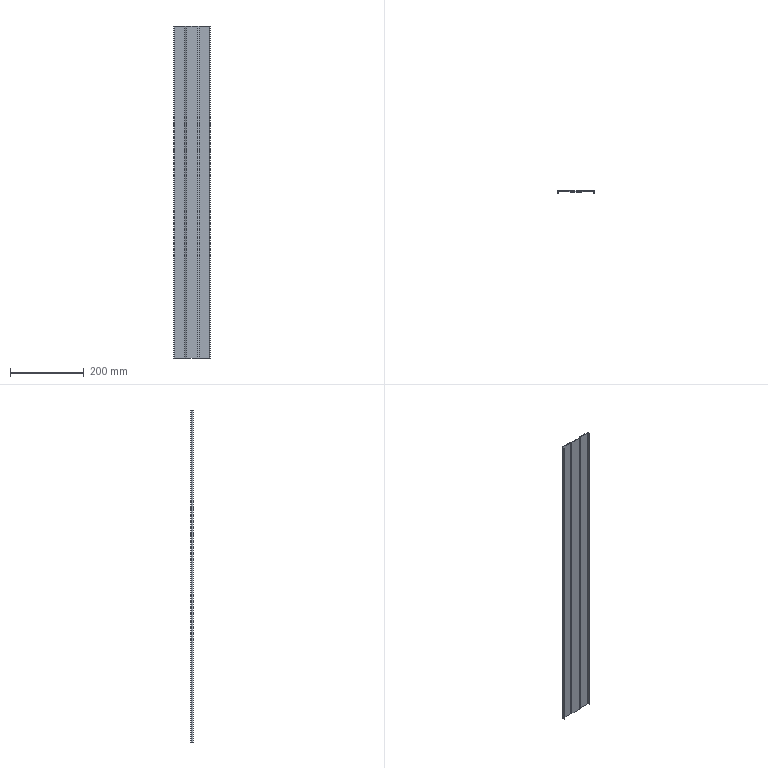Part | STEP file | Crossbeam front guard plate | 1 solid | 54 faces | box 98 x 8 x 898 mm | volume 149433 mm3 | plane 42 | cylinder 12 | commonest cylinder face diameters 1 x6 4 x6
STEP:
#1=CARTESIAN_POINT('',(98.,-2.,898.));
#2=VERTEX_POINT('',#1);
#3=CARTESIAN_POINT('',(96.5,-2.,898.));
#4=VERTEX_POINT('',#3);
#5=CARTESIAN_POINT('',(98.,-2.,898.));
#6=DIRECTION('',(-1.,0.,0.));
#7=VECTOR('',#6,1000.);
#8=LINE('',#5,#7);
#9=EDGE_CURVE('',#2,#4,#8,.T.);
#10=ORIENTED_EDGE('',*,*,#9,.F.);
#11=CARTESIAN_POINT('',(96.,0.,898.));
#12=VERTEX_POINT('',#11);
#13=CARTESIAN_POINT('',(96.,-2.,898.));
#14=DIRECTION('',(0.,0.,1.));
#15=DIRECTION('',(-1.,0.,0.));
#16=AXIS2_PLACEMENT_3D('',#13,#14,#15);
#17=CIRCLE('',#16,2.);
#18=EDGE_CURVE('',#2,#12,#17,.T.);
#19=ORIENTED_EDGE('',*,*,#18,.T.);
#20=CARTESIAN_POINT('',(96.,-1.5,898.));
#21=VERTEX_POINT('',#20);
#22=CARTESIAN_POINT('',(96.,-1.5,898.));
#23=DIRECTION('',(0.,1.,0.));
#24=VECTOR('',#23,1000.);
#25=LINE('',#22,#24);
#26=EDGE_CURVE('',#21,#12,#25,.T.);
#27=ORIENTED_EDGE('',*,*,#26,.F.);
#28=CARTESIAN_POINT('',(96.,-2.,898.));
#29=DIRECTION('',(0.,0.,1.));
#30=DIRECTION('',(1.,0.,0.));
#31=AXIS2_PLACEMENT_3D('',#28,#29,#30);
#32=CIRCLE('',#31,0.5);
#33=EDGE_CURVE('',#4,#21,#32,.T.);
#34=ORIENTED_EDGE('',*,*,#33,.F.);
#35=EDGE_LOOP('',(#10,#19,#27,#34));
#36=FACE_OUTER_BOUND('',#35,.T.);
#37=CARTESIAN_POINT('',(98.,-2.,898.));
#38=DIRECTION('',(0.,0.,1.));
#39=DIRECTION('',(1.,0.,0.));
#40=AXIS2_PLACEMENT_3D('',#37,#38,#39);
#41=PLANE('',#40);
#42=ADVANCED_FACE('',(#36),#41,.T.);
#43=CARTESIAN_POINT('',(98.,-8.,898.));
#44=VERTEX_POINT('',#43);
#45=CARTESIAN_POINT('',(98.,0.,898.));
#46=DIRECTION('',(0.,1.,0.));
#47=VECTOR('',#46,1000.);
#48=LINE('',#45,#47);
#49=EDGE_CURVE('',#44,#2,#48,.T.);
#50=ORIENTED_EDGE('',*,*,#49,.T.);
#51=ORIENTED_EDGE('',*,*,#9,.T.);
#52=CARTESIAN_POINT('',(96.5,-8.,898.));
#53=VERTEX_POINT('',#52);
#54=CARTESIAN_POINT('',(96.5,0.,898.));
#55=DIRECTION('',(0.,1.,0.));
#56=VECTOR('',#55,1000.);
#57=LINE('',#54,#56);
#58=EDGE_CURVE('',#53,#4,#57,.T.);
#59=ORIENTED_EDGE('',*,*,#58,.F.);
#60=CARTESIAN_POINT('',(98.,-8.,898.));
#61=DIRECTION('',(-1.,0.,0.));
#62=VECTOR('',#61,1000.);
#63=LINE('',#60,#62);
#64=EDGE_CURVE('',#44,#53,#63,.T.);
#65=ORIENTED_EDGE('',*,*,#64,.F.);
#66=EDGE_LOOP('',(#50,#51,#59,#65));
#67=FACE_OUTER_BOUND('',#66,.T.);
#68=CARTESIAN_POINT('',(96.,-1.5,898.));
#69=DIRECTION('',(0.,0.,1.));
#70=DIRECTION('',(1.,0.,0.));
#71=AXIS2_PLACEMENT_3D('',#68,#69,#70);
#72=PLANE('',#71);
#73=ADVANCED_FACE('',(#67),#72,.T.);
#74=CARTESIAN_POINT('',(96.,0.,0.));
#75=VERTEX_POINT('',#74);
#76=CARTESIAN_POINT('',(96.,-1.5,0.));
#77=VERTEX_POINT('',#76);
#78=CARTESIAN_POINT('',(96.,0.,0.));
#79=DIRECTION('',(0.,-1.,0.));
#80=VECTOR('',#79,1000.);
#81=LINE('',#78,#80);
#82=EDGE_CURVE('',#75,#77,#81,.T.);
#83=ORIENTED_EDGE('',*,*,#82,.F.);
#84=CARTESIAN_POINT('',(98.,-2.,0.));
#85=VERTEX_POINT('',#84);
#86=CARTESIAN_POINT('',(96.,-2.,0.));
#87=DIRECTION('',(0.,0.,1.));
#88=DIRECTION('',(-1.,0.,0.));
#89=AXIS2_PLACEMENT_3D('',#86,#87,#88);
#90=CIRCLE('',#89,2.);
#91=EDGE_CURVE('',#85,#75,#90,.T.);
#92=ORIENTED_EDGE('',*,*,#91,.F.);
#93=CARTESIAN_POINT('',(96.5,-2.,0.));
#94=VERTEX_POINT('',#93);
#95=CARTESIAN_POINT('',(96.5,-2.,0.));
#96=DIRECTION('',(1.,0.,0.));
#97=VECTOR('',#96,1000.);
#98=LINE('',#95,#97);
#99=EDGE_CURVE('',#94,#85,#98,.T.);
#100=ORIENTED_EDGE('',*,*,#99,.F.);
#101=CARTESIAN_POINT('',(96.,-2.,0.));
#102=DIRECTION('',(0.,0.,1.));
#103=DIRECTION('',(1.,0.,0.));
#104=AXIS2_PLACEMENT_3D('',#101,#102,#103);
#105=CIRCLE('',#104,0.5);
#106=EDGE_CURVE('',#94,#77,#105,.T.);
#107=ORIENTED_EDGE('',*,*,#106,.T.);
#108=EDGE_LOOP('',(#83,#92,#100,#107));
#109=FACE_OUTER_BOUND('',#108,.T.);
#110=CARTESIAN_POINT('',(96.,0.,0.));
#111=DIRECTION('',(0.,0.,-1.));
#112=DIRECTION('',(-1.,0.,0.));
#113=AXIS2_PLACEMENT_3D('',#110,#111,#112);
#114=PLANE('',#113);
#115=ADVANCED_FACE('',(#109),#114,.T.);
#116=CARTESIAN_POINT('',(68.,0.,0.));
#117=VERTEX_POINT('',#116);
#118=CARTESIAN_POINT('',(67.464,0.,0.));
#119=DIRECTION('',(-1.,0.,0.));
#120=VECTOR('',#119,1000.);
#121=LINE('',#118,#120);
#122=EDGE_CURVE('',#75,#117,#121,.T.);
#123=ORIENTED_EDGE('',*,*,#122,.F.);
#124=ORIENTED_EDGE('',*,*,#82,.T.);
#125=CARTESIAN_POINT('',(68.,-1.5,0.));
#126=VERTEX_POINT('',#125);
#127=CARTESIAN_POINT('',(67.464,-1.5,0.));
#128=DIRECTION('',(-1.,0.,0.));
#129=VECTOR('',#128,1000.);
#130=LINE('',#127,#129);
#131=EDGE_CURVE('',#77,#126,#130,.T.);
#132=ORIENTED_EDGE('',*,*,#131,.T.);
#133=CARTESIAN_POINT('',(68.,-1.5,0.));
#134=DIRECTION('',(0.,1.,0.));
#135=VECTOR('',#134,1000.);
#136=LINE('',#133,#135);
#137=EDGE_CURVE('',#126,#117,#136,.T.);
#138=ORIENTED_EDGE('',*,*,#137,.T.);
#139=EDGE_LOOP('',(#123,#124,#132,#138));
#140=FACE_OUTER_BOUND('',#139,.T.);
#141=CARTESIAN_POINT('',(96.5,-2.,0.));
#142=DIRECTION('',(0.,0.,-1.));
#143=DIRECTION('',(-1.,0.,0.));
#144=AXIS2_PLACEMENT_3D('',#141,#142,#143);
#145=PLANE('',#144);
#146=ADVANCED_FACE('',(#140),#145,.T.);
#147=CARTESIAN_POINT('',(68.,0.,898.));
#148=VERTEX_POINT('',#147);
#149=CARTESIAN_POINT('',(68.,-1.5,898.));
#150=VERTEX_POINT('',#149);
#151=CARTESIAN_POINT('',(68.,0.,898.));
#152=DIRECTION('',(0.,-1.,0.));
#153=VECTOR('',#152,1000.);
#154=LINE('',#151,#153);
#155=EDGE_CURVE('',#148,#150,#154,.T.);
#156=ORIENTED_EDGE('',*,*,#155,.F.);
#157=CARTESIAN_POINT('',(67.,-0.2679,898.));
#158=VERTEX_POINT('',#157);
#159=CARTESIAN_POINT('',(68.,-2.,898.));
#160=DIRECTION('',(0.,0.,1.));
#161=DIRECTION('',(-1.,0.,0.));
#162=AXIS2_PLACEMENT_3D('',#159,#160,#161);
#163=CIRCLE('',#162,2.);
#164=EDGE_CURVE('',#148,#158,#163,.T.);
#165=ORIENTED_EDGE('',*,*,#164,.T.);
#166=CARTESIAN_POINT('',(67.75,-1.567,898.));
#167=VERTEX_POINT('',#166);
#168=CARTESIAN_POINT('',(67.75,-1.567,898.));
#169=DIRECTION('',(-0.5,0.866,0.));
#170=VECTOR('',#169,1000.);
#171=LINE('',#168,#170);
#172=EDGE_CURVE('',#167,#158,#171,.T.);
#173=ORIENTED_EDGE('',*,*,#172,.F.);
#174=CARTESIAN_POINT('',(68.,-2.,898.));
#175=DIRECTION('',(0.,0.,1.));
#176=DIRECTION('',(1.,0.,0.));
#177=AXIS2_PLACEMENT_3D('',#174,#175,#176);
#178=CIRCLE('',#177,0.5);
#179=EDGE_CURVE('',#150,#167,#178,.T.);
#180=ORIENTED_EDGE('',*,*,#179,.F.);
#181=EDGE_LOOP('',(#156,#165,#173,#180));
#182=FACE_OUTER_BOUND('',#181,.T.);
#183=CARTESIAN_POINT('',(68.,0.,898.));
#184=DIRECTION('',(0.,0.,1.));
#185=DIRECTION('',(1.,0.,0.));
#186=AXIS2_PLACEMENT_3D('',#183,#184,#185);
#187=PLANE('',#186);
#188=ADVANCED_FACE('',(#182),#187,.T.);
#189=CARTESIAN_POINT('',(67.464,0.,898.));
#190=DIRECTION('',(-1.,0.,0.));
#191=VECTOR('',#190,1000.);
#192=LINE('',#189,#191);
#193=EDGE_CURVE('',#12,#148,#192,.T.);
#194=ORIENTED_EDGE('',*,*,#193,.T.);
#195=ORIENTED_EDGE('',*,*,#155,.T.);
#196=CARTESIAN_POINT('',(67.464,-1.5,898.));
#197=DIRECTION('',(-1.,0.,0.));
#198=VECTOR('',#197,1000.);
#199=LINE('',#196,#198);
#200=EDGE_CURVE('',#21,#150,#199,.T.);
#201=ORIENTED_EDGE('',*,*,#200,.F.);
#202=ORIENTED_EDGE('',*,*,#26,.T.);
#203=EDGE_LOOP('',(#194,#195,#201,#202));
#204=FACE_OUTER_BOUND('',#203,.T.);
#205=CARTESIAN_POINT('',(67.75,-1.567,898.));
#206=DIRECTION('',(0.,0.,1.));
#207=DIRECTION('',(1.,0.,0.));
#208=AXIS2_PLACEMENT_3D('',#205,#206,#207);
#209=PLANE('',#208);
#210=ADVANCED_FACE('',(#204),#209,.T.);
#211=CARTESIAN_POINT('',(67.,-0.2679,0.));
#212=VERTEX_POINT('',#211);
#213=CARTESIAN_POINT('',(67.75,-1.567,0.));
#214=VERTEX_POINT('',#213);
#215=CARTESIAN_POINT('',(67.,-0.2679,0.));
#216=DIRECTION('',(0.5,-0.866,0.));
#217=VECTOR('',#216,1000.);
#218=LINE('',#215,#217);
#219=EDGE_CURVE('',#212,#214,#218,.T.);
#220=ORIENTED_EDGE('',*,*,#219,.F.);
#221=CARTESIAN_POINT('',(68.,-2.,0.));
#222=DIRECTION('',(0.,0.,1.));
#223=DIRECTION('',(-1.,0.,0.));
#224=AXIS2_PLACEMENT_3D('',#221,#222,#223);
#225=CIRCLE('',#224,2.);
#226=EDGE_CURVE('',#117,#212,#225,.T.);
#227=ORIENTED_EDGE('',*,*,#226,.F.);
#228=ORIENTED_EDGE('',*,*,#137,.F.);
#229=CARTESIAN_POINT('',(68.,-2.,0.));
#230=DIRECTION('',(0.,0.,1.));
#231=DIRECTION('',(1.,0.,0.));
#232=AXIS2_PLACEMENT_3D('',#229,#230,#231);
#233=CIRCLE('',#232,0.5);
#234=EDGE_CURVE('',#126,#214,#233,.T.);
#235=ORIENTED_EDGE('',*,*,#234,.T.);
#236=EDGE_LOOP('',(#220,#227,#228,#235));
#237=FACE_OUTER_BOUND('',#236,.T.);
#238=CARTESIAN_POINT('',(67.,-0.2679,0.));
#239=DIRECTION('',(0.,0.,-1.));
#240=DIRECTION('',(-1.,0.,0.));
#241=AXIS2_PLACEMENT_3D('',#238,#239,#240);
#242=PLANE('',#241);
#243=ADVANCED_FACE('',(#237),#242,.T.);
#244=CARTESIAN_POINT('',(64.116,-1.933,0.));
#245=VERTEX_POINT('',#244);
#246=CARTESIAN_POINT('',(64.,-2.,0.));
#247=DIRECTION('',(-0.866,-0.5,0.));
#248=VECTOR('',#247,1000.);
#249=LINE('',#246,#248);
#250=EDGE_CURVE('',#212,#245,#249,.T.);
#251=ORIENTED_EDGE('',*,*,#250,.F.);
#252=ORIENTED_EDGE('',*,*,#219,.T.);
#253=CARTESIAN_POINT('',(64.866,-3.232,0.));
#254=VERTEX_POINT('',#253);
#255=CARTESIAN_POINT('',(64.75,-3.299,0.));
#256=DIRECTION('',(-0.866,-0.5,0.));
#257=VECTOR('',#256,1000.);
#258=LINE('',#255,#257);
#259=EDGE_CURVE('',#214,#254,#258,.T.);
#260=ORIENTED_EDGE('',*,*,#259,.T.);
#261=CARTESIAN_POINT('',(64.866,-3.232,0.));
#262=DIRECTION('',(-0.5,0.866,0.));
#263=VECTOR('',#262,1000.);
#264=LINE('',#261,#263);
#265=EDGE_CURVE('',#254,#245,#264,.T.);
#266=ORIENTED_EDGE('',*,*,#265,.T.);
#267=EDGE_LOOP('',(#251,#252,#260,#266));
#268=FACE_OUTER_BOUND('',#267,.T.);
#269=CARTESIAN_POINT('',(68.,-1.5,0.));
#270=DIRECTION('',(0.,0.,-1.));
#271=DIRECTION('',(-1.,0.,0.));
#272=AXIS2_PLACEMENT_3D('',#269,#270,#271);
#273=PLANE('',#272);
#274=ADVANCED_FACE('',(#268),#273,.T.);
#275=CARTESIAN_POINT('',(64.116,-1.933,898.));
#276=VERTEX_POINT('',#275);
#277=CARTESIAN_POINT('',(64.866,-3.232,898.));
#278=VERTEX_POINT('',#277);
#279=CARTESIAN_POINT('',(64.116,-1.933,898.));
#280=DIRECTION('',(0.5,-0.866,0.));
#281=VECTOR('',#280,1000.);
#282=LINE('',#279,#281);
#283=EDGE_CURVE('',#276,#278,#282,.T.);
#284=ORIENTED_EDGE('',*,*,#283,.F.);
#285=CARTESIAN_POINT('',(63.866,-2.,898.));
#286=VERTEX_POINT('',#285);
#287=CARTESIAN_POINT('',(63.866,-1.5,898.));
#288=DIRECTION('',(0.,0.,-1.));
#289=DIRECTION('',(1.,0.,0.));
#290=AXIS2_PLACEMENT_3D('',#287,#288,#289);
#291=CIRCLE('',#290,0.5);
#292=EDGE_CURVE('',#276,#286,#291,.T.);
#293=ORIENTED_EDGE('',*,*,#292,.T.);
#294=CARTESIAN_POINT('',(63.866,-3.5,898.));
#295=VERTEX_POINT('',#294);
#296=CARTESIAN_POINT('',(63.866,-3.5,898.));
#297=DIRECTION('',(0.,1.,0.));
#298=VECTOR('',#297,1000.);
#299=LINE('',#296,#298);
#300=EDGE_CURVE('',#295,#286,#299,.T.);
#301=ORIENTED_EDGE('',*,*,#300,.F.);
#302=CARTESIAN_POINT('',(63.866,-1.5,898.));
#303=DIRECTION('',(0.,0.,-1.));
#304=DIRECTION('',(1.,0.,0.));
#305=AXIS2_PLACEMENT_3D('',#302,#303,#304);
#306=CIRCLE('',#305,2.);
#307=EDGE_CURVE('',#278,#295,#306,.T.);
#308=ORIENTED_EDGE('',*,*,#307,.F.);
#309=EDGE_LOOP('',(#284,#293,#301,#308));
#310=FACE_OUTER_BOUND('',#309,.T.);
#311=CARTESIAN_POINT('',(64.116,-1.933,898.));
#312=DIRECTION('',(0.,0.,1.));
#313=DIRECTION('',(1.,0.,0.));
#314=AXIS2_PLACEMENT_3D('',#311,#312,#313);
#315=PLANE('',#314);
#316=ADVANCED_FACE('',(#310),#315,.T.);
#317=CARTESIAN_POINT('',(64.,-2.,898.));
#318=DIRECTION('',(-0.866,-0.5,0.));
#319=VECTOR('',#318,1000.);
#320=LINE('',#317,#319);
#321=EDGE_CURVE('',#158,#276,#320,.T.);
#322=ORIENTED_EDGE('',*,*,#321,.T.);
#323=ORIENTED_EDGE('',*,*,#283,.T.);
#324=CARTESIAN_POINT('',(64.75,-3.299,898.));
#325=DIRECTION('',(-0.866,-0.5,0.));
#326=VECTOR('',#325,1000.);
#327=LINE('',#324,#326);
#328=EDGE_CURVE('',#167,#278,#327,.T.);
#329=ORIENTED_EDGE('',*,*,#328,.F.);
#330=ORIENTED_EDGE('',*,*,#172,.T.);
#331=EDGE_LOOP('',(#322,#323,#329,#330));
#332=FACE_OUTER_BOUND('',#331,.T.);
#333=CARTESIAN_POINT('',(63.866,-3.5,898.));
#334=DIRECTION('',(0.,0.,1.));
#335=DIRECTION('',(1.,0.,0.));
#336=AXIS2_PLACEMENT_3D('',#333,#334,#335);
#337=PLANE('',#336);
#338=ADVANCED_FACE('',(#332),#337,.T.);
#339=CARTESIAN_POINT('',(63.866,-2.,0.));
#340=VERTEX_POINT('',#339);
#341=CARTESIAN_POINT('',(63.866,-3.5,0.));
#342=VERTEX_POINT('',#341);
#343=CARTESIAN_POINT('',(63.866,-2.,0.));
#344=DIRECTION('',(0.,-1.,0.));
#345=VECTOR('',#344,1000.);
#346=LINE('',#343,#345);
#347=EDGE_CURVE('',#340,#342,#346,.T.);
#348=ORIENTED_EDGE('',*,*,#347,.F.);
#349=CARTESIAN_POINT('',(63.866,-1.5,0.));
#350=DIRECTION('',(0.,0.,-1.));
#351=DIRECTION('',(1.,0.,0.));
#352=AXIS2_PLACEMENT_3D('',#349,#350,#351);
#353=CIRCLE('',#352,0.5);
#354=EDGE_CURVE('',#245,#340,#353,.T.);
#355=ORIENTED_EDGE('',*,*,#354,.F.);
#356=ORIENTED_EDGE('',*,*,#265,.F.);
#357=CARTESIAN_POINT('',(63.866,-1.5,0.));
#358=DIRECTION('',(0.,0.,-1.));
#359=DIRECTION('',(1.,0.,0.));
#360=AXIS2_PLACEMENT_3D('',#357,#358,#359);
#361=CIRCLE('',#360,2.);
#362=EDGE_CURVE('',#254,#342,#361,.T.);
#363=ORIENTED_EDGE('',*,*,#362,.T.);
#364=EDGE_LOOP('',(#348,#355,#356,#363));
#365=FACE_OUTER_BOUND('',#364,.T.);
#366=CARTESIAN_POINT('',(63.866,-2.,0.));
#367=DIRECTION('',(0.,0.,-1.));
#368=DIRECTION('',(-1.,0.,0.));
#369=AXIS2_PLACEMENT_3D('',#366,#367,#368);
#370=PLANE('',#369);
#371=ADVANCED_FACE('',(#365),#370,.T.);
#372=CARTESIAN_POINT('',(34.134,-2.,0.));
#373=VERTEX_POINT('',#372);
#374=CARTESIAN_POINT('',(34.,-2.,0.));
#375=DIRECTION('',(-1.,0.,0.));
#376=VECTOR('',#375,1000.);
#377=LINE('',#374,#376);
#378=EDGE_CURVE('',#340,#373,#377,.T.);
#379=ORIENTED_EDGE('',*,*,#378,.F.);
#380=ORIENTED_EDGE('',*,*,#347,.T.);
#381=CARTESIAN_POINT('',(34.134,-3.5,0.));
#382=VERTEX_POINT('',#381);
#383=CARTESIAN_POINT('',(34.,-3.5,0.));
#384=DIRECTION('',(-1.,0.,0.));
#385=VECTOR('',#384,1000.);
#386=LINE('',#383,#385);
#387=EDGE_CURVE('',#342,#382,#386,.T.);
#388=ORIENTED_EDGE('',*,*,#387,.T.);
#389=CARTESIAN_POINT('',(34.134,-3.5,0.));
#390=DIRECTION('',(0.,1.,0.));
#391=VECTOR('',#390,1000.);
#392=LINE('',#389,#391);
#393=EDGE_CURVE('',#382,#373,#392,.T.);
#394=ORIENTED_EDGE('',*,*,#393,.T.);
#395=EDGE_LOOP('',(#379,#380,#388,#394));
#396=FACE_OUTER_BOUND('',#395,.T.);
#397=CARTESIAN_POINT('',(64.866,-3.232,0.));
#398=DIRECTION('',(0.,0.,-1.));
#399=DIRECTION('',(-1.,0.,0.));
#400=AXIS2_PLACEMENT_3D('',#397,#398,#399);
#401=PLANE('',#400);
#402=ADVANCED_FACE('',(#396),#401,.T.);
#403=CARTESIAN_POINT('',(34.134,-2.,898.));
#404=VERTEX_POINT('',#403);
#405=CARTESIAN_POINT('',(34.134,-3.5,898.));
#406=VERTEX_POINT('',#405);
#407=CARTESIAN_POINT('',(34.134,-2.,898.));
#408=DIRECTION('',(0.,-1.,0.));
#409=VECTOR('',#408,1000.);
#410=LINE('',#407,#409);
#411=EDGE_CURVE('',#404,#406,#410,.T.);
#412=ORIENTED_EDGE('',*,*,#411,.F.);
#413=CARTESIAN_POINT('',(33.884,-1.933,898.));
#414=VERTEX_POINT('',#413);
#415=CARTESIAN_POINT('',(34.134,-1.5,898.));
#416=DIRECTION('',(0.,0.,-1.));
#417=DIRECTION('',(1.,0.,0.));
#418=AXIS2_PLACEMENT_3D('',#415,#416,#417);
#419=CIRCLE('',#418,0.5);
#420=EDGE_CURVE('',#404,#414,#419,.T.);
#421=ORIENTED_EDGE('',*,*,#420,.T.);
#422=CARTESIAN_POINT('',(33.134,-3.232,898.));
#423=VERTEX_POINT('',#422);
#424=CARTESIAN_POINT('',(33.134,-3.232,898.));
#425=DIRECTION('',(0.5,0.866,0.));
#426=VECTOR('',#425,1000.);
#427=LINE('',#424,#426);
#428=EDGE_CURVE('',#423,#414,#427,.T.);
#429=ORIENTED_EDGE('',*,*,#428,.F.);
#430=CARTESIAN_POINT('',(34.134,-1.5,898.));
#431=DIRECTION('',(0.,0.,-1.));
#432=DIRECTION('',(1.,0.,0.));
#433=AXIS2_PLACEMENT_3D('',#430,#431,#432);
#434=CIRCLE('',#433,2.);
#435=EDGE_CURVE('',#406,#423,#434,.T.);
#436=ORIENTED_EDGE('',*,*,#435,.F.);
#437=EDGE_LOOP('',(#412,#421,#429,#436));
#438=FACE_OUTER_BOUND('',#437,.T.);
#439=CARTESIAN_POINT('',(34.134,-2.,898.));
#440=DIRECTION('',(0.,0.,1.));
#441=DIRECTION('',(1.,0.,0.));
#442=AXIS2_PLACEMENT_3D('',#439,#440,#441);
#443=PLANE('',#442);
#444=ADVANCED_FACE('',(#438),#443,.T.);
#445=CARTESIAN_POINT('',(34.,-2.,898.));
#446=DIRECTION('',(-1.,0.,0.));
#447=VECTOR('',#446,1000.);
#448=LINE('',#445,#447);
#449=EDGE_CURVE('',#286,#404,#448,.T.);
#450=ORIENTED_EDGE('',*,*,#449,.T.);
#451=ORIENTED_EDGE('',*,*,#411,.T.);
#452=CARTESIAN_POINT('',(34.,-3.5,898.));
#453=DIRECTION('',(-1.,0.,0.));
#454=VECTOR('',#453,1000.);
#455=LINE('',#452,#454);
#456=EDGE_CURVE('',#295,#406,#455,.T.);
#457=ORIENTED_EDGE('',*,*,#456,.F.);
#458=ORIENTED_EDGE('',*,*,#300,.T.);
#459=EDGE_LOOP('',(#450,#451,#457,#458));
#460=FACE_OUTER_BOUND('',#459,.T.);
#461=CARTESIAN_POINT('',(33.134,-3.232,898.));
#462=DIRECTION('',(0.,0.,1.));
#463=DIRECTION('',(1.,0.,0.));
#464=AXIS2_PLACEMENT_3D('',#461,#462,#463);
#465=PLANE('',#464);
#466=ADVANCED_FACE('',(#460),#465,.T.);
#467=CARTESIAN_POINT('',(33.884,-1.933,0.));
#468=VERTEX_POINT('',#467);
#469=CARTESIAN_POINT('',(33.134,-3.232,0.));
#470=VERTEX_POINT('',#469);
#471=CARTESIAN_POINT('',(33.884,-1.933,0.));
#472=DIRECTION('',(-0.5,-0.866,0.));
#473=VECTOR('',#472,1000.);
#474=LINE('',#471,#473);
#475=EDGE_CURVE('',#468,#470,#474,.T.);
#476=ORIENTED_EDGE('',*,*,#475,.F.);
#477=CARTESIAN_POINT('',(34.134,-1.5,0.));
#478=DIRECTION('',(0.,0.,-1.));
#479=DIRECTION('',(1.,0.,0.));
#480=AXIS2_PLACEMENT_3D('',#477,#478,#479);
#481=CIRCLE('',#480,0.5);
#482=EDGE_CURVE('',#373,#468,#481,.T.);
#483=ORIENTED_EDGE('',*,*,#482,.F.);
#484=ORIENTED_EDGE('',*,*,#393,.F.);
#485=CARTESIAN_POINT('',(34.134,-1.5,0.));
#486=DIRECTION('',(0.,0.,-1.));
#487=DIRECTION('',(1.,0.,0.));
#488=AXIS2_PLACEMENT_3D('',#485,#486,#487);
#489=CIRCLE('',#488,2.);
#490=EDGE_CURVE('',#382,#470,#489,.T.);
#491=ORIENTED_EDGE('',*,*,#490,.T.);
#492=EDGE_LOOP('',(#476,#483,#484,#491));
#493=FACE_OUTER_BOUND('',#492,.T.);
#494=CARTESIAN_POINT('',(33.884,-1.933,0.));
#495=DIRECTION('',(0.,0.,-1.));
#496=DIRECTION('',(-1.,0.,0.));
#497=AXIS2_PLACEMENT_3D('',#494,#495,#496);
#498=PLANE('',#497);
#499=ADVANCED_FACE('',(#493),#498,.T.);
#500=CARTESIAN_POINT('',(31.,-0.2679,0.));
#501=VERTEX_POINT('',#500);
#502=CARTESIAN_POINT('',(30.536,0.,0.));
#503=DIRECTION('',(-0.866,0.5,0.));
#504=VECTOR('',#503,1000.);
#505=LINE('',#502,#504);
#506=EDGE_CURVE('',#468,#501,#505,.T.);
#507=ORIENTED_EDGE('',*,*,#506,.F.);
#508=ORIENTED_EDGE('',*,*,#475,.T.);
#509=CARTESIAN_POINT('',(30.25,-1.567,0.));
#510=VERTEX_POINT('',#509);
#511=CARTESIAN_POINT('',(29.786,-1.299,0.));
#512=DIRECTION('',(-0.866,0.5,0.));
#513=VECTOR('',#512,1000.);
#514=LINE('',#511,#513);
#515=EDGE_CURVE('',#470,#510,#514,.T.);
#516=ORIENTED_EDGE('',*,*,#515,.T.);
#517=CARTESIAN_POINT('',(30.25,-1.567,0.));
#518=DIRECTION('',(0.5,0.866,0.));
#519=VECTOR('',#518,1000.);
#520=LINE('',#517,#519);
#521=EDGE_CURVE('',#510,#501,#520,.T.);
#522=ORIENTED_EDGE('',*,*,#521,.T.);
#523=EDGE_LOOP('',(#507,#508,#516,#522));
#524=FACE_OUTER_BOUND('',#523,.T.);
#525=CARTESIAN_POINT('',(34.134,-3.5,0.));
#526=DIRECTION('',(0.,0.,-1.));
#527=DIRECTION('',(-1.,0.,0.));
#528=AXIS2_PLACEMENT_3D('',#525,#526,#527);
#529=PLANE('',#528);
#530=ADVANCED_FACE('',(#524),#529,.T.);
#531=CARTESIAN_POINT('',(31.,-0.2679,898.));
#532=VERTEX_POINT('',#531);
#533=CARTESIAN_POINT('',(30.25,-1.567,898.));
#534=VERTEX_POINT('',#533);
#535=CARTESIAN_POINT('',(31.,-0.2679,898.));
#536=DIRECTION('',(-0.5,-0.866,0.));
#537=VECTOR('',#536,1000.);
#538=LINE('',#535,#537);
#539=EDGE_CURVE('',#532,#534,#538,.T.);
#540=ORIENTED_EDGE('',*,*,#539,.F.);
#541=CARTESIAN_POINT('',(30.,0.,898.));
#542=VERTEX_POINT('',#541);
#543=CARTESIAN_POINT('',(30.,-2.,898.));
#544=DIRECTION('',(0.,0.,1.));
#545=DIRECTION('',(-1.,0.,0.));
#546=AXIS2_PLACEMENT_3D('',#543,#544,#545);
#547=CIRCLE('',#546,2.);
#548=EDGE_CURVE('',#532,#542,#547,.T.);
#549=ORIENTED_EDGE('',*,*,#548,.T.);
#550=CARTESIAN_POINT('',(30.,-1.5,898.));
#551=VERTEX_POINT('',#550);
#552=CARTESIAN_POINT('',(30.,-1.5,898.));
#553=DIRECTION('',(0.,1.,0.));
#554=VECTOR('',#553,1000.);
#555=LINE('',#552,#554);
#556=EDGE_CURVE('',#551,#542,#555,.T.);
#557=ORIENTED_EDGE('',*,*,#556,.F.);
#558=CARTESIAN_POINT('',(30.,-2.,898.));
#559=DIRECTION('',(0.,0.,1.));
#560=DIRECTION('',(1.,0.,0.));
#561=AXIS2_PLACEMENT_3D('',#558,#559,#560);
#562=CIRCLE('',#561,0.5);
#563=EDGE_CURVE('',#534,#551,#562,.T.);
#564=ORIENTED_EDGE('',*,*,#563,.F.);
#565=EDGE_LOOP('',(#540,#549,#557,#564));
#566=FACE_OUTER_BOUND('',#565,.T.);
#567=CARTESIAN_POINT('',(31.,-0.2679,898.));
#568=DIRECTION('',(0.,0.,1.));
#569=DIRECTION('',(1.,0.,0.));
#570=AXIS2_PLACEMENT_3D('',#567,#568,#569);
#571=PLANE('',#570);
#572=ADVANCED_FACE('',(#566),#571,.T.);
#573=CARTESIAN_POINT('',(30.536,0.,898.));
#574=DIRECTION('',(-0.866,0.5,0.));
#575=VECTOR('',#574,1000.);
#576=LINE('',#573,#575);
#577=EDGE_CURVE('',#414,#532,#576,.T.);
#578=ORIENTED_EDGE('',*,*,#577,.T.);
#579=ORIENTED_EDGE('',*,*,#539,.T.);
#580=CARTESIAN_POINT('',(29.786,-1.299,898.));
#581=DIRECTION('',(-0.866,0.5,0.));
#582=VECTOR('',#581,1000.);
#583=LINE('',#580,#582);
#584=EDGE_CURVE('',#423,#534,#583,.T.);
#585=ORIENTED_EDGE('',*,*,#584,.F.);
#586=ORIENTED_EDGE('',*,*,#428,.T.);
#587=EDGE_LOOP('',(#578,#579,#585,#586));
#588=FACE_OUTER_BOUND('',#587,.T.);
#589=CARTESIAN_POINT('',(30.,-1.5,898.));
#590=DIRECTION('',(0.,0.,1.));
#591=DIRECTION('',(1.,0.,0.));
#592=AXIS2_PLACEMENT_3D('',#589,#590,#591);
#593=PLANE('',#592);
#594=ADVANCED_FACE('',(#588),#593,.T.);
#595=CARTESIAN_POINT('',(30.,0.,0.));
#596=VERTEX_POINT('',#595);
#597=CARTESIAN_POINT('',(30.,-1.5,0.));
#598=VERTEX_POINT('',#597);
#599=CARTESIAN_POINT('',(30.,0.,0.));
#600=DIRECTION('',(0.,-1.,0.));
#601=VECTOR('',#600,1000.);
#602=LINE('',#599,#601);
#603=EDGE_CURVE('',#596,#598,#602,.T.);
#604=ORIENTED_EDGE('',*,*,#603,.F.);
#605=CARTESIAN_POINT('',(30.,-2.,0.));
#606=DIRECTION('',(0.,0.,1.));
#607=DIRECTION('',(-1.,0.,0.));
#608=AXIS2_PLACEMENT_3D('',#605,#606,#607);
#609=CIRCLE('',#608,2.);
#610=EDGE_CURVE('',#501,#596,#609,.T.);
#611=ORIENTED_EDGE('',*,*,#610,.F.);
#612=ORIENTED_EDGE('',*,*,#521,.F.);
#613=CARTESIAN_POINT('',(30.,-2.,0.));
#614=DIRECTION('',(0.,0.,1.));
#615=DIRECTION('',(1.,0.,0.));
#616=AXIS2_PLACEMENT_3D('',#613,#614,#615);
#617=CIRCLE('',#616,0.5);
#618=EDGE_CURVE('',#510,#598,#617,.T.);
#619=ORIENTED_EDGE('',*,*,#618,.T.);
#620=EDGE_LOOP('',(#604,#611,#612,#619));
#621=FACE_OUTER_BOUND('',#620,.T.);
#622=CARTESIAN_POINT('',(30.,0.,0.));
#623=DIRECTION('',(0.,0.,-1.));
#624=DIRECTION('',(-1.,0.,0.));
#625=AXIS2_PLACEMENT_3D('',#622,#623,#624);
#626=PLANE('',#625);
#627=ADVANCED_FACE('',(#621),#626,.T.);
#628=CARTESIAN_POINT('',(2.,0.,0.));
#629=VERTEX_POINT('',#628);
#630=CARTESIAN_POINT('',(0.,0.,0.));
#631=DIRECTION('',(-1.,0.,0.));
#632=VECTOR('',#631,1000.);
#633=LINE('',#630,#632);
#634=EDGE_CURVE('',#596,#629,#633,.T.);
#635=ORIENTED_EDGE('',*,*,#634,.F.);
#636=ORIENTED_EDGE('',*,*,#603,.T.);
#637=CARTESIAN_POINT('',(2.,-1.5,0.));
#638=VERTEX_POINT('',#637);
#639=CARTESIAN_POINT('',(0.,-1.5,0.));
#640=DIRECTION('',(-1.,0.,0.));
#641=VECTOR('',#640,1000.);
#642=LINE('',#639,#641);
#643=EDGE_CURVE('',#598,#638,#642,.T.);
#644=ORIENTED_EDGE('',*,*,#643,.T.);
#645=CARTESIAN_POINT('',(2.,-1.5,0.));
#646=DIRECTION('',(0.,1.,0.));
#647=VECTOR('',#646,1000.);
#648=LINE('',#645,#647);
#649=EDGE_CURVE('',#638,#629,#648,.T.);
#650=ORIENTED_EDGE('',*,*,#649,.T.);
#651=EDGE_LOOP('',(#635,#636,#644,#650));
#652=FACE_OUTER_BOUND('',#651,.T.);
#653=CARTESIAN_POINT('',(30.25,-1.567,0.));
#654=DIRECTION('',(0.,0.,-1.));
#655=DIRECTION('',(-1.,0.,0.));
#656=AXIS2_PLACEMENT_3D('',#653,#654,#655);
#657=PLANE('',#656);
#658=ADVANCED_FACE('',(#652),#657,.T.);
#659=CARTESIAN_POINT('',(2.,0.,898.));
#660=VERTEX_POINT('',#659);
#661=CARTESIAN_POINT('',(2.,-1.5,898.));
#662=VERTEX_POINT('',#661);
#663=CARTESIAN_POINT('',(2.,0.,898.));
#664=DIRECTION('',(0.,-1.,0.));
#665=VECTOR('',#664,1000.);
#666=LINE('',#663,#665);
#667=EDGE_CURVE('',#660,#662,#666,.T.);
#668=ORIENTED_EDGE('',*,*,#667,.F.);
#669=CARTESIAN_POINT('',(0.,-2.,898.));
#670=VERTEX_POINT('',#669);
#671=CARTESIAN_POINT('',(2.,-2.,898.));
#672=DIRECTION('',(0.,0.,1.));
#673=DIRECTION('',(-1.,0.,0.));
#674=AXIS2_PLACEMENT_3D('',#671,#672,#673);
#675=CIRCLE('',#674,2.);
#676=EDGE_CURVE('',#660,#670,#675,.T.);
#677=ORIENTED_EDGE('',*,*,#676,.T.);
#678=CARTESIAN_POINT('',(1.5,-2.,898.));
#679=VERTEX_POINT('',#678);
#680=CARTESIAN_POINT('',(1.5,-2.,898.));
#681=DIRECTION('',(-1.,0.,0.));
#682=VECTOR('',#681,1000.);
#683=LINE('',#680,#682);
#684=EDGE_CURVE('',#679,#670,#683,.T.);
#685=ORIENTED_EDGE('',*,*,#684,.F.);
#686=CARTESIAN_POINT('',(2.,-2.,898.));
#687=DIRECTION('',(0.,0.,1.));
#688=DIRECTION('',(1.,0.,0.));
#689=AXIS2_PLACEMENT_3D('',#686,#687,#688);
#690=CIRCLE('',#689,0.5);
#691=EDGE_CURVE('',#662,#679,#690,.T.);
#692=ORIENTED_EDGE('',*,*,#691,.F.);
#693=EDGE_LOOP('',(#668,#677,#685,#692));
#694=FACE_OUTER_BOUND('',#693,.T.);
#695=CARTESIAN_POINT('',(2.,0.,898.));
#696=DIRECTION('',(0.,0.,1.));
#697=DIRECTION('',(1.,0.,0.));
#698=AXIS2_PLACEMENT_3D('',#695,#696,#697);
#699=PLANE('',#698);
#700=ADVANCED_FACE('',(#694),#699,.T.);
#701=CARTESIAN_POINT('',(0.,0.,898.));
#702=DIRECTION('',(-1.,0.,0.));
#703=VECTOR('',#702,1000.);
#704=LINE('',#701,#703);
#705=EDGE_CURVE('',#542,#660,#704,.T.);
#706=ORIENTED_EDGE('',*,*,#705,.T.);
#707=ORIENTED_EDGE('',*,*,#667,.T.);
#708=CARTESIAN_POINT('',(0.,-1.5,898.));
#709=DIRECTION('',(-1.,0.,0.));
#710=VECTOR('',#709,1000.);
#711=LINE('',#708,#710);
#712=EDGE_CURVE('',#551,#662,#711,.T.);
#713=ORIENTED_EDGE('',*,*,#712,.F.);
#714=ORIENTED_EDGE('',*,*,#556,.T.);
#715=EDGE_LOOP('',(#706,#707,#713,#714));
#716=FACE_OUTER_BOUND('',#715,.T.);
#717=CARTESIAN_POINT('',(1.5,-2.,898.));
#718=DIRECTION('',(0.,0.,1.));
#719=DIRECTION('',(1.,0.,0.));
#720=AXIS2_PLACEMENT_3D('',#717,#718,#719);
#721=PLANE('',#720);
#722=ADVANCED_FACE('',(#716),#721,.T.);
#723=CARTESIAN_POINT('',(0.,-2.,0.));
#724=VERTEX_POINT('',#723);
#725=CARTESIAN_POINT('',(1.5,-2.,0.));
#726=VERTEX_POINT('',#725);
#727=CARTESIAN_POINT('',(0.,-2.,0.));
#728=DIRECTION('',(1.,0.,0.));
#729=VECTOR('',#728,1000.);
#730=LINE('',#727,#729);
#731=EDGE_CURVE('',#724,#726,#730,.T.);
#732=ORIENTED_EDGE('',*,*,#731,.F.);
#733=CARTESIAN_POINT('',(2.,-2.,0.));
#734=DIRECTION('',(0.,0.,1.));
#735=DIRECTION('',(-1.,0.,0.));
#736=AXIS2_PLACEMENT_3D('',#733,#734,#735);
#737=CIRCLE('',#736,2.);
#738=EDGE_CURVE('',#629,#724,#737,.T.);
#739=ORIENTED_EDGE('',*,*,#738,.F.);
#740=ORIENTED_EDGE('',*,*,#649,.F.);
#741=CARTESIAN_POINT('',(2.,-2.,0.));
#742=DIRECTION('',(0.,0.,1.));
#743=DIRECTION('',(1.,0.,0.));
#744=AXIS2_PLACEMENT_3D('',#741,#742,#743);
#745=CIRCLE('',#744,0.5);
#746=EDGE_CURVE('',#638,#726,#745,.T.);
#747=ORIENTED_EDGE('',*,*,#746,.T.);
#748=EDGE_LOOP('',(#732,#739,#740,#747));
#749=FACE_OUTER_BOUND('',#748,.T.);
#750=CARTESIAN_POINT('',(0.,-2.,0.));
#751=DIRECTION('',(0.,0.,-1.));
#752=DIRECTION('',(-1.,0.,0.));
#753=AXIS2_PLACEMENT_3D('',#750,#751,#752);
#754=PLANE('',#753);
#755=ADVANCED_FACE('',(#749),#754,.T.);
#756=CARTESIAN_POINT('',(0.,-8.,0.));
#757=VERTEX_POINT('',#756);
#758=CARTESIAN_POINT('',(0.,0.,0.));
#759=DIRECTION('',(0.,-1.,0.));
#760=VECTOR('',#759,1000.);
#761=LINE('',#758,#760);
#762=EDGE_CURVE('',#724,#757,#761,.T.);
#763=ORIENTED_EDGE('',*,*,#762,.F.);
#764=ORIENTED_EDGE('',*,*,#731,.T.);
#765=CARTESIAN_POINT('',(1.5,-8.,0.));
#766=VERTEX_POINT('',#765);
#767=CARTESIAN_POINT('',(1.5,0.,0.));
#768=DIRECTION('',(0.,-1.,0.));
#769=VECTOR('',#768,1000.);
#770=LINE('',#767,#769);
#771=EDGE_CURVE('',#726,#766,#770,.T.);
#772=ORIENTED_EDGE('',*,*,#771,.T.);
#773=CARTESIAN_POINT('',(1.5,-8.,0.));
#774=DIRECTION('',(-1.,0.,0.));
#775=VECTOR('',#774,1000.);
#776=LINE('',#773,#775);
#777=EDGE_CURVE('',#766,#757,#776,.T.);
#778=ORIENTED_EDGE('',*,*,#777,.T.);
#779=EDGE_LOOP('',(#763,#764,#772,#778));
#780=FACE_OUTER_BOUND('',#779,.T.);
#781=CARTESIAN_POINT('',(2.,-1.5,0.));
#782=DIRECTION('',(0.,0.,-1.));
#783=DIRECTION('',(-1.,0.,0.));
#784=AXIS2_PLACEMENT_3D('',#781,#782,#783);
#785=PLANE('',#784);
#786=ADVANCED_FACE('',(#780),#785,.T.);
#787=ORIENTED_EDGE('',*,*,#762,.T.);
#788=CARTESIAN_POINT('',(0.,-8.,898.));
#789=VERTEX_POINT('',#788);
#790=CARTESIAN_POINT('',(0.,-8.,898.));
#791=DIRECTION('',(0.,0.,-1.));
#792=VECTOR('',#791,1000.);
#793=LINE('',#790,#792);
#794=EDGE_CURVE('',#789,#757,#793,.T.);
#795=ORIENTED_EDGE('',*,*,#794,.F.);
#796=CARTESIAN_POINT('',(0.,0.,898.));
#797=DIRECTION('',(0.,-1.,0.));
#798=VECTOR('',#797,1000.);
#799=LINE('',#796,#798);
#800=EDGE_CURVE('',#670,#789,#799,.T.);
#801=ORIENTED_EDGE('',*,*,#800,.F.);
#802=CARTESIAN_POINT('',(0.,-2.,898.));
#803=DIRECTION('',(0.,0.,-1.));
#804=VECTOR('',#803,1000.);
#805=LINE('',#802,#804);
#806=EDGE_CURVE('',#670,#724,#805,.T.);
#807=ORIENTED_EDGE('',*,*,#806,.T.);
#808=EDGE_LOOP('',(#787,#795,#801,#807));
#809=FACE_OUTER_BOUND('',#808,.T.);
#810=CARTESIAN_POINT('',(0.,0.,898.));
#811=DIRECTION('',(1.,0.,0.));
#812=DIRECTION('',(0.,1.,0.));
#813=AXIS2_PLACEMENT_3D('',#810,#811,#812);
#814=PLANE('',#813);
#815=ADVANCED_FACE('',(#809),#814,.F.);
#816=ORIENTED_EDGE('',*,*,#777,.F.);
#817=CARTESIAN_POINT('',(1.5,-8.,898.));
#818=VERTEX_POINT('',#817);
#819=CARTESIAN_POINT('',(1.5,-8.,898.));
#820=DIRECTION('',(0.,0.,-1.));
#821=VECTOR('',#820,1000.);
#822=LINE('',#819,#821);
#823=EDGE_CURVE('',#818,#766,#822,.T.);
#824=ORIENTED_EDGE('',*,*,#823,.F.);
#825=CARTESIAN_POINT('',(1.5,-8.,898.));
#826=DIRECTION('',(-1.,0.,0.));
#827=VECTOR('',#826,1000.);
#828=LINE('',#825,#827);
#829=EDGE_CURVE('',#818,#789,#828,.T.);
#830=ORIENTED_EDGE('',*,*,#829,.T.);
#831=ORIENTED_EDGE('',*,*,#794,.T.);
#832=EDGE_LOOP('',(#816,#824,#830,#831));
#833=FACE_OUTER_BOUND('',#832,.T.);
#834=CARTESIAN_POINT('',(1.5,-8.,898.));
#835=DIRECTION('',(0.,-1.,0.));
#836=DIRECTION('',(0.,0.,-1.));
#837=AXIS2_PLACEMENT_3D('',#834,#835,#836);
#838=PLANE('',#837);
#839=ADVANCED_FACE('',(#833),#838,.T.);
#840=ORIENTED_EDGE('',*,*,#771,.F.);
#841=CARTESIAN_POINT('',(1.5,-2.,898.));
#842=DIRECTION('',(0.,0.,-1.));
#843=VECTOR('',#842,1000.);
#844=LINE('',#841,#843);
#845=EDGE_CURVE('',#679,#726,#844,.T.);
#846=ORIENTED_EDGE('',*,*,#845,.F.);
#847=CARTESIAN_POINT('',(1.5,0.,898.));
#848=DIRECTION('',(0.,-1.,0.));
#849=VECTOR('',#848,1000.);
#850=LINE('',#847,#849);
#851=EDGE_CURVE('',#679,#818,#850,.T.);
#852=ORIENTED_EDGE('',*,*,#851,.T.);
#853=ORIENTED_EDGE('',*,*,#823,.T.);
#854=EDGE_LOOP('',(#840,#846,#852,#853));
#855=FACE_OUTER_BOUND('',#854,.T.);
#856=CARTESIAN_POINT('',(1.5,0.,898.));
#857=DIRECTION('',(1.,0.,0.));
#858=DIRECTION('',(0.,1.,0.));
#859=AXIS2_PLACEMENT_3D('',#856,#857,#858);
#860=PLANE('',#859);
#861=ADVANCED_FACE('',(#855),#860,.T.);
#862=ORIENTED_EDGE('',*,*,#746,.F.);
#863=CARTESIAN_POINT('',(2.,-1.5,898.));
#864=DIRECTION('',(0.,0.,-1.));
#865=VECTOR('',#864,1000.);
#866=LINE('',#863,#865);
#867=EDGE_CURVE('',#662,#638,#866,.T.);
#868=ORIENTED_EDGE('',*,*,#867,.F.);
#869=ORIENTED_EDGE('',*,*,#691,.T.);
#870=ORIENTED_EDGE('',*,*,#845,.T.);
#871=EDGE_LOOP('',(#862,#868,#869,#870));
#872=FACE_OUTER_BOUND('',#871,.T.);
#873=CARTESIAN_POINT('',(2.,-2.,898.));
#874=DIRECTION('',(0.,0.,-1.));
#875=DIRECTION('',(-1.,0.,0.));
#876=AXIS2_PLACEMENT_3D('',#873,#874,#875);
#877=CYLINDRICAL_SURFACE('',#876,0.5);
#878=ADVANCED_FACE('',(#872),#877,.F.);
#879=ORIENTED_EDGE('',*,*,#643,.F.);
#880=CARTESIAN_POINT('',(30.,-1.5,898.));
#881=DIRECTION('',(0.,0.,-1.));
#882=VECTOR('',#881,1000.);
#883=LINE('',#880,#882);
#884=EDGE_CURVE('',#551,#598,#883,.T.);
#885=ORIENTED_EDGE('',*,*,#884,.F.);
#886=ORIENTED_EDGE('',*,*,#712,.T.);
#887=ORIENTED_EDGE('',*,*,#867,.T.);
#888=EDGE_LOOP('',(#879,#885,#886,#887));
#889=FACE_OUTER_BOUND('',#888,.T.);
#890=CARTESIAN_POINT('',(0.,-1.5,898.));
#891=DIRECTION('',(0.,-1.,0.));
#892=DIRECTION('',(0.,0.,-1.));
#893=AXIS2_PLACEMENT_3D('',#890,#891,#892);
#894=PLANE('',#893);
#895=ADVANCED_FACE('',(#889),#894,.T.);
#896=ORIENTED_EDGE('',*,*,#618,.F.);
#897=CARTESIAN_POINT('',(30.25,-1.567,898.));
#898=DIRECTION('',(0.,0.,-1.));
#899=VECTOR('',#898,1000.);
#900=LINE('',#897,#899);
#901=EDGE_CURVE('',#534,#510,#900,.T.);
#902=ORIENTED_EDGE('',*,*,#901,.F.);
#903=ORIENTED_EDGE('',*,*,#563,.T.);
#904=ORIENTED_EDGE('',*,*,#884,.T.);
#905=EDGE_LOOP('',(#896,#902,#903,#904));
#906=FACE_OUTER_BOUND('',#905,.T.);
#907=CARTESIAN_POINT('',(30.,-2.,898.));
#908=DIRECTION('',(0.,0.,-1.));
#909=DIRECTION('',(-1.,0.,0.));
#910=AXIS2_PLACEMENT_3D('',#907,#908,#909);
#911=CYLINDRICAL_SURFACE('',#910,0.5);
#912=ADVANCED_FACE('',(#906),#911,.F.);
#913=ORIENTED_EDGE('',*,*,#515,.F.);
#914=CARTESIAN_POINT('',(33.134,-3.232,898.));
#915=DIRECTION('',(0.,0.,-1.));
#916=VECTOR('',#915,1000.);
#917=LINE('',#914,#916);
#918=EDGE_CURVE('',#423,#470,#917,.T.);
#919=ORIENTED_EDGE('',*,*,#918,.F.);
#920=ORIENTED_EDGE('',*,*,#584,.T.);
#921=ORIENTED_EDGE('',*,*,#901,.T.);
#922=EDGE_LOOP('',(#913,#919,#920,#921));
#923=FACE_OUTER_BOUND('',#922,.T.);
#924=CARTESIAN_POINT('',(29.786,-1.299,898.));
#925=DIRECTION('',(-0.5,-0.866,0.));
#926=DIRECTION('',(0.866,-0.5,0.));
#927=AXIS2_PLACEMENT_3D('',#924,#925,#926);
#928=PLANE('',#927);
#929=ADVANCED_FACE('',(#923),#928,.T.);
#930=ORIENTED_EDGE('',*,*,#490,.F.);
#931=CARTESIAN_POINT('',(34.134,-3.5,898.));
#932=DIRECTION('',(0.,0.,-1.));
#933=VECTOR('',#932,1000.);
#934=LINE('',#931,#933);
#935=EDGE_CURVE('',#406,#382,#934,.T.);
#936=ORIENTED_EDGE('',*,*,#935,.F.);
#937=ORIENTED_EDGE('',*,*,#435,.T.);
#938=ORIENTED_EDGE('',*,*,#918,.T.);
#939=EDGE_LOOP('',(#930,#936,#937,#938));
#940=FACE_OUTER_BOUND('',#939,.T.);
#941=CARTESIAN_POINT('',(34.134,-1.5,898.));
#942=DIRECTION('',(0.,0.,-1.));
#943=DIRECTION('',(-1.,0.,0.));
#944=AXIS2_PLACEMENT_3D('',#941,#942,#943);
#945=CYLINDRICAL_SURFACE('',#944,2.);
#946=ADVANCED_FACE('',(#940),#945,.T.);
#947=ORIENTED_EDGE('',*,*,#387,.F.);
#948=CARTESIAN_POINT('',(63.866,-3.5,898.));
#949=DIRECTION('',(0.,0.,-1.));
#950=VECTOR('',#949,1000.);
#951=LINE('',#948,#950);
#952=EDGE_CURVE('',#295,#342,#951,.T.);
#953=ORIENTED_EDGE('',*,*,#952,.F.);
#954=ORIENTED_EDGE('',*,*,#456,.T.);
#955=ORIENTED_EDGE('',*,*,#935,.T.);
#956=EDGE_LOOP('',(#947,#953,#954,#955));
#957=FACE_OUTER_BOUND('',#956,.T.);
#958=CARTESIAN_POINT('',(34.,-3.5,898.));
#959=DIRECTION('',(0.,-1.,0.));
#960=DIRECTION('',(1.,0.,0.));
#961=AXIS2_PLACEMENT_3D('',#958,#959,#960);
#962=PLANE('',#961);
#963=ADVANCED_FACE('',(#957),#962,.T.);
#964=ORIENTED_EDGE('',*,*,#362,.F.);
#965=CARTESIAN_POINT('',(64.866,-3.232,898.));
#966=DIRECTION('',(0.,0.,-1.));
#967=VECTOR('',#966,1000.);
#968=LINE('',#965,#967);
#969=EDGE_CURVE('',#278,#254,#968,.T.);
#970=ORIENTED_EDGE('',*,*,#969,.F.);
#971=ORIENTED_EDGE('',*,*,#307,.T.);
#972=ORIENTED_EDGE('',*,*,#952,.T.);
#973=EDGE_LOOP('',(#964,#970,#971,#972));
#974=FACE_OUTER_BOUND('',#973,.T.);
#975=CARTESIAN_POINT('',(63.866,-1.5,898.));
#976=DIRECTION('',(0.,0.,-1.));
#977=DIRECTION('',(-1.,0.,0.));
#978=AXIS2_PLACEMENT_3D('',#975,#976,#977);
#979=CYLINDRICAL_SURFACE('',#978,2.);
#980=ADVANCED_FACE('',(#974),#979,.T.);
#981=ORIENTED_EDGE('',*,*,#259,.F.);
#982=CARTESIAN_POINT('',(67.75,-1.567,898.));
#983=DIRECTION('',(0.,0.,-1.));
#984=VECTOR('',#983,1000.);
#985=LINE('',#982,#984);
#986=EDGE_CURVE('',#167,#214,#985,.T.);
#987=ORIENTED_EDGE('',*,*,#986,.F.);
#988=ORIENTED_EDGE('',*,*,#328,.T.);
#989=ORIENTED_EDGE('',*,*,#969,.T.);
#990=EDGE_LOOP('',(#981,#987,#988,#989));
#991=FACE_OUTER_BOUND('',#990,.T.);
#992=CARTESIAN_POINT('',(64.75,-3.299,898.));
#993=DIRECTION('',(0.5,-0.866,0.));
#994=DIRECTION('',(0.866,0.5,0.));
#995=AXIS2_PLACEMENT_3D('',#992,#993,#994);
#996=PLANE('',#995);
#997=ADVANCED_FACE('',(#991),#996,.T.);
#998=ORIENTED_EDGE('',*,*,#234,.F.);
#999=CARTESIAN_POINT('',(68.,-1.5,898.));
#1000=DIRECTION('',(0.,0.,-1.));
#1001=VECTOR('',#1000,1000.);
#1002=LINE('',#999,#1001);
#1003=EDGE_CURVE('',#150,#126,#1002,.T.);
#1004=ORIENTED_EDGE('',*,*,#1003,.F.);
#1005=ORIENTED_EDGE('',*,*,#179,.T.);
#1006=ORIENTED_EDGE('',*,*,#986,.T.);
#1007=EDGE_LOOP('',(#998,#1004,#1005,#1006));
#1008=FACE_OUTER_BOUND('',#1007,.T.);
#1009=CARTESIAN_POINT('',(68.,-2.,898.));
#1010=DIRECTION('',(0.,0.,-1.));
#1011=DIRECTION('',(-1.,0.,0.));
#1012=AXIS2_PLACEMENT_3D('',#1009,#1010,#1011);
#1013=CYLINDRICAL_SURFACE('',#1012,0.5);
#1014=ADVANCED_FACE('',(#1008),#1013,.F.);
#1015=ORIENTED_EDGE('',*,*,#131,.F.);
#1016=CARTESIAN_POINT('',(96.,-1.5,898.));
#1017=DIRECTION('',(0.,0.,-1.));
#1018=VECTOR('',#1017,1000.);
#1019=LINE('',#1016,#1018);
#1020=EDGE_CURVE('',#21,#77,#1019,.T.);
#1021=ORIENTED_EDGE('',*,*,#1020,.F.);
#1022=ORIENTED_EDGE('',*,*,#200,.T.);
#1023=ORIENTED_EDGE('',*,*,#1003,.T.);
#1024=EDGE_LOOP('',(#1015,#1021,#1022,#1023));
#1025=FACE_OUTER_BOUND('',#1024,.T.);
#1026=CARTESIAN_POINT('',(67.464,-1.5,898.));
#1027=DIRECTION('',(0.,-1.,0.));
#1028=DIRECTION('',(1.,0.,0.));
#1029=AXIS2_PLACEMENT_3D('',#1026,#1027,#1028);
#1030=PLANE('',#1029);
#1031=ADVANCED_FACE('',(#1025),#1030,.T.);
#1032=ORIENTED_EDGE('',*,*,#106,.F.);
#1033=CARTESIAN_POINT('',(96.5,-2.,898.));
#1034=DIRECTION('',(0.,0.,-1.));
#1035=VECTOR('',#1034,1000.);
#1036=LINE('',#1033,#1035);
#1037=EDGE_CURVE('',#4,#94,#1036,.T.);
#1038=ORIENTED_EDGE('',*,*,#1037,.F.);
#1039=ORIENTED_EDGE('',*,*,#33,.T.);
#1040=ORIENTED_EDGE('',*,*,#1020,.T.);
#1041=EDGE_LOOP('',(#1032,#1038,#1039,#1040));
#1042=FACE_OUTER_BOUND('',#1041,.T.);
#1043=CARTESIAN_POINT('',(96.,-2.,898.));
#1044=DIRECTION('',(0.,0.,-1.));
#1045=DIRECTION('',(-1.,0.,0.));
#1046=AXIS2_PLACEMENT_3D('',#1043,#1044,#1045);
#1047=CYLINDRICAL_SURFACE('',#1046,0.5);
#1048=ADVANCED_FACE('',(#1042),#1047,.F.);
#1049=CARTESIAN_POINT('',(96.5,-8.,0.));
#1050=VERTEX_POINT('',#1049);
#1051=CARTESIAN_POINT('',(96.5,0.,0.));
#1052=DIRECTION('',(0.,1.,0.));
#1053=VECTOR('',#1052,1000.);
#1054=LINE('',#1051,#1053);
#1055=EDGE_CURVE('',#1050,#94,#1054,.T.);
#1056=ORIENTED_EDGE('',*,*,#1055,.F.);
#1057=CARTESIAN_POINT('',(96.5,-8.,898.));
#1058=DIRECTION('',(0.,0.,-1.));
#1059=VECTOR('',#1058,1000.);
#1060=LINE('',#1057,#1059);
#1061=EDGE_CURVE('',#53,#1050,#1060,.T.);
#1062=ORIENTED_EDGE('',*,*,#1061,.F.);
#1063=ORIENTED_EDGE('',*,*,#58,.T.);
#1064=ORIENTED_EDGE('',*,*,#1037,.T.);
#1065=EDGE_LOOP('',(#1056,#1062,#1063,#1064));
#1066=FACE_OUTER_BOUND('',#1065,.T.);
#1067=CARTESIAN_POINT('',(96.5,0.,898.));
#1068=DIRECTION('',(-1.,0.,0.));
#1069=DIRECTION('',(0.,0.,1.));
#1070=AXIS2_PLACEMENT_3D('',#1067,#1068,#1069);
#1071=PLANE('',#1070);
#1072=ADVANCED_FACE('',(#1066),#1071,.T.);
#1073=CARTESIAN_POINT('',(98.,-8.,0.));
#1074=VERTEX_POINT('',#1073);
#1075=CARTESIAN_POINT('',(98.,-8.,0.));
#1076=DIRECTION('',(-1.,0.,0.));
#1077=VECTOR('',#1076,1000.);
#1078=LINE('',#1075,#1077);
#1079=EDGE_CURVE('',#1074,#1050,#1078,.T.);
#1080=ORIENTED_EDGE('',*,*,#1079,.F.);
#1081=CARTESIAN_POINT('',(98.,-8.,898.));
#1082=DIRECTION('',(0.,0.,-1.));
#1083=VECTOR('',#1082,1000.);
#1084=LINE('',#1081,#1083);
#1085=EDGE_CURVE('',#44,#1074,#1084,.T.);
#1086=ORIENTED_EDGE('',*,*,#1085,.F.);
#1087=ORIENTED_EDGE('',*,*,#64,.T.);
#1088=ORIENTED_EDGE('',*,*,#1061,.T.);
#1089=EDGE_LOOP('',(#1080,#1086,#1087,#1088));
#1090=FACE_OUTER_BOUND('',#1089,.T.);
#1091=CARTESIAN_POINT('',(98.,-8.,898.));
#1092=DIRECTION('',(0.,-1.,0.));
#1093=DIRECTION('',(0.,0.,-1.));
#1094=AXIS2_PLACEMENT_3D('',#1091,#1092,#1093);
#1095=PLANE('',#1094);
#1096=ADVANCED_FACE('',(#1090),#1095,.T.);
#1097=CARTESIAN_POINT('',(98.,0.,0.));
#1098=DIRECTION('',(0.,1.,0.));
#1099=VECTOR('',#1098,1000.);
#1100=LINE('',#1097,#1099);
#1101=EDGE_CURVE('',#1074,#85,#1100,.T.);
#1102=ORIENTED_EDGE('',*,*,#1101,.T.);
#1103=CARTESIAN_POINT('',(98.,-2.,898.));
#1104=DIRECTION('',(0.,0.,-1.));
#1105=VECTOR('',#1104,1000.);
#1106=LINE('',#1103,#1105);
#1107=EDGE_CURVE('',#2,#85,#1106,.T.);
#1108=ORIENTED_EDGE('',*,*,#1107,.F.);
#1109=ORIENTED_EDGE('',*,*,#49,.F.);
#1110=ORIENTED_EDGE('',*,*,#1085,.T.);
#1111=EDGE_LOOP('',(#1102,#1108,#1109,#1110));
#1112=FACE_OUTER_BOUND('',#1111,.T.);
#1113=CARTESIAN_POINT('',(98.,0.,898.));
#1114=DIRECTION('',(-1.,0.,0.));
#1115=DIRECTION('',(0.,0.,1.));
#1116=AXIS2_PLACEMENT_3D('',#1113,#1114,#1115);
#1117=PLANE('',#1116);
#1118=ADVANCED_FACE('',(#1112),#1117,.F.);
#1119=ORIENTED_EDGE('',*,*,#91,.T.);
#1120=CARTESIAN_POINT('',(96.,0.,898.));
#1121=DIRECTION('',(0.,0.,-1.));
#1122=VECTOR('',#1121,1000.);
#1123=LINE('',#1120,#1122);
#1124=EDGE_CURVE('',#12,#75,#1123,.T.);
#1125=ORIENTED_EDGE('',*,*,#1124,.F.);
#1126=ORIENTED_EDGE('',*,*,#18,.F.);
#1127=ORIENTED_EDGE('',*,*,#1107,.T.);
#1128=EDGE_LOOP('',(#1119,#1125,#1126,#1127));
#1129=FACE_OUTER_BOUND('',#1128,.T.);
#1130=CARTESIAN_POINT('',(96.,-2.,898.));
#1131=DIRECTION('',(0.,0.,-1.));
#1132=DIRECTION('',(-1.,0.,0.));
#1133=AXIS2_PLACEMENT_3D('',#1130,#1131,#1132);
#1134=CYLINDRICAL_SURFACE('',#1133,2.);
#1135=ADVANCED_FACE('',(#1129),#1134,.T.);
#1136=ORIENTED_EDGE('',*,*,#122,.T.);
#1137=CARTESIAN_POINT('',(68.,0.,898.));
#1138=DIRECTION('',(0.,0.,-1.));
#1139=VECTOR('',#1138,1000.);
#1140=LINE('',#1137,#1139);
#1141=EDGE_CURVE('',#148,#117,#1140,.T.);
#1142=ORIENTED_EDGE('',*,*,#1141,.F.);
#1143=ORIENTED_EDGE('',*,*,#193,.F.);
#1144=ORIENTED_EDGE('',*,*,#1124,.T.);
#1145=EDGE_LOOP('',(#1136,#1142,#1143,#1144));
#1146=FACE_OUTER_BOUND('',#1145,.T.);
#1147=CARTESIAN_POINT('',(67.464,0.,898.));
#1148=DIRECTION('',(0.,-1.,0.));
#1149=DIRECTION('',(1.,0.,0.));
#1150=AXIS2_PLACEMENT_3D('',#1147,#1148,#1149);
#1151=PLANE('',#1150);
#1152=ADVANCED_FACE('',(#1146),#1151,.F.);
#1153=ORIENTED_EDGE('',*,*,#226,.T.);
#1154=CARTESIAN_POINT('',(67.,-0.2679,898.));
#1155=DIRECTION('',(0.,0.,-1.));
#1156=VECTOR('',#1155,1000.);
#1157=LINE('',#1154,#1156);
#1158=EDGE_CURVE('',#158,#212,#1157,.T.);
#1159=ORIENTED_EDGE('',*,*,#1158,.F.);
#1160=ORIENTED_EDGE('',*,*,#164,.F.);
#1161=ORIENTED_EDGE('',*,*,#1141,.T.);
#1162=EDGE_LOOP('',(#1153,#1159,#1160,#1161));
#1163=FACE_OUTER_BOUND('',#1162,.T.);
#1164=CARTESIAN_POINT('',(68.,-2.,898.));
#1165=DIRECTION('',(0.,0.,-1.));
#1166=DIRECTION('',(-1.,0.,0.));
#1167=AXIS2_PLACEMENT_3D('',#1164,#1165,#1166);
#1168=CYLINDRICAL_SURFACE('',#1167,2.);
#1169=ADVANCED_FACE('',(#1163),#1168,.T.);
#1170=ORIENTED_EDGE('',*,*,#250,.T.);
#1171=CARTESIAN_POINT('',(64.116,-1.933,898.));
#1172=DIRECTION('',(0.,0.,-1.));
#1173=VECTOR('',#1172,1000.);
#1174=LINE('',#1171,#1173);
#1175=EDGE_CURVE('',#276,#245,#1174,.T.);
#1176=ORIENTED_EDGE('',*,*,#1175,.F.);
#1177=ORIENTED_EDGE('',*,*,#321,.F.);
#1178=ORIENTED_EDGE('',*,*,#1158,.T.);
#1179=EDGE_LOOP('',(#1170,#1176,#1177,#1178));
#1180=FACE_OUTER_BOUND('',#1179,.T.);
#1181=CARTESIAN_POINT('',(64.,-2.,898.));
#1182=DIRECTION('',(0.5,-0.866,0.));
#1183=DIRECTION('',(0.866,0.5,0.));
#1184=AXIS2_PLACEMENT_3D('',#1181,#1182,#1183);
#1185=PLANE('',#1184);
#1186=ADVANCED_FACE('',(#1180),#1185,.F.);
#1187=ORIENTED_EDGE('',*,*,#354,.T.);
#1188=CARTESIAN_POINT('',(63.866,-2.,898.));
#1189=DIRECTION('',(0.,0.,-1.));
#1190=VECTOR('',#1189,1000.);
#1191=LINE('',#1188,#1190);
#1192=EDGE_CURVE('',#286,#340,#1191,.T.);
#1193=ORIENTED_EDGE('',*,*,#1192,.F.);
#1194=ORIENTED_EDGE('',*,*,#292,.F.);
#1195=ORIENTED_EDGE('',*,*,#1175,.T.);
#1196=EDGE_LOOP('',(#1187,#1193,#1194,#1195));
#1197=FACE_OUTER_BOUND('',#1196,.T.);
#1198=CARTESIAN_POINT('',(63.866,-1.5,898.));
#1199=DIRECTION('',(0.,0.,-1.));
#1200=DIRECTION('',(-1.,0.,0.));
#1201=AXIS2_PLACEMENT_3D('',#1198,#1199,#1200);
#1202=CYLINDRICAL_SURFACE('',#1201,0.5);
#1203=ADVANCED_FACE('',(#1197),#1202,.F.);
#1204=ORIENTED_EDGE('',*,*,#378,.T.);
#1205=CARTESIAN_POINT('',(34.134,-2.,898.));
#1206=DIRECTION('',(0.,0.,-1.));
#1207=VECTOR('',#1206,1000.);
#1208=LINE('',#1205,#1207);
#1209=EDGE_CURVE('',#404,#373,#1208,.T.);
#1210=ORIENTED_EDGE('',*,*,#1209,.F.);
#1211=ORIENTED_EDGE('',*,*,#449,.F.);
#1212=ORIENTED_EDGE('',*,*,#1192,.T.);
#1213=EDGE_LOOP('',(#1204,#1210,#1211,#1212));
#1214=FACE_OUTER_BOUND('',#1213,.T.);
#1215=CARTESIAN_POINT('',(34.,-2.,898.));
#1216=DIRECTION('',(0.,-1.,0.));
#1217=DIRECTION('',(1.,0.,0.));
#1218=AXIS2_PLACEMENT_3D('',#1215,#1216,#1217);
#1219=PLANE('',#1218);
#1220=ADVANCED_FACE('',(#1214),#1219,.F.);
#1221=ORIENTED_EDGE('',*,*,#482,.T.);
#1222=CARTESIAN_POINT('',(33.884,-1.933,898.));
#1223=DIRECTION('',(0.,0.,-1.));
#1224=VECTOR('',#1223,1000.);
#1225=LINE('',#1222,#1224);
#1226=EDGE_CURVE('',#414,#468,#1225,.T.);
#1227=ORIENTED_EDGE('',*,*,#1226,.F.);
#1228=ORIENTED_EDGE('',*,*,#420,.F.);
#1229=ORIENTED_EDGE('',*,*,#1209,.T.);
#1230=EDGE_LOOP('',(#1221,#1227,#1228,#1229));
#1231=FACE_OUTER_BOUND('',#1230,.T.);
#1232=CARTESIAN_POINT('',(34.134,-1.5,898.));
#1233=DIRECTION('',(0.,0.,-1.));
#1234=DIRECTION('',(-1.,0.,0.));
#1235=AXIS2_PLACEMENT_3D('',#1232,#1233,#1234);
#1236=CYLINDRICAL_SURFACE('',#1235,0.5);
#1237=ADVANCED_FACE('',(#1231),#1236,.F.);
#1238=ORIENTED_EDGE('',*,*,#506,.T.);
#1239=CARTESIAN_POINT('',(31.,-0.2679,898.));
#1240=DIRECTION('',(0.,0.,-1.));
#1241=VECTOR('',#1240,1000.);
#1242=LINE('',#1239,#1241);
#1243=EDGE_CURVE('',#532,#501,#1242,.T.);
#1244=ORIENTED_EDGE('',*,*,#1243,.F.);
#1245=ORIENTED_EDGE('',*,*,#577,.F.);
#1246=ORIENTED_EDGE('',*,*,#1226,.T.);
#1247=EDGE_LOOP('',(#1238,#1244,#1245,#1246));
#1248=FACE_OUTER_BOUND('',#1247,.T.);
#1249=CARTESIAN_POINT('',(30.536,0.,898.));
#1250=DIRECTION('',(-0.5,-0.866,0.));
#1251=DIRECTION('',(0.866,-0.5,0.));
#1252=AXIS2_PLACEMENT_3D('',#1249,#1250,#1251);
#1253=PLANE('',#1252);
#1254=ADVANCED_FACE('',(#1248),#1253,.F.);
#1255=ORIENTED_EDGE('',*,*,#610,.T.);
#1256=CARTESIAN_POINT('',(30.,0.,898.));
#1257=DIRECTION('',(0.,0.,-1.));
#1258=VECTOR('',#1257,1000.);
#1259=LINE('',#1256,#1258);
#1260=EDGE_CURVE('',#542,#596,#1259,.T.);
#1261=ORIENTED_EDGE('',*,*,#1260,.F.);
#1262=ORIENTED_EDGE('',*,*,#548,.F.);
#1263=ORIENTED_EDGE('',*,*,#1243,.T.);
#1264=EDGE_LOOP('',(#1255,#1261,#1262,#1263));
#1265=FACE_OUTER_BOUND('',#1264,.T.);
#1266=CARTESIAN_POINT('',(30.,-2.,898.));
#1267=DIRECTION('',(0.,0.,-1.));
#1268=DIRECTION('',(-1.,0.,0.));
#1269=AXIS2_PLACEMENT_3D('',#1266,#1267,#1268);
#1270=CYLINDRICAL_SURFACE('',#1269,2.);
#1271=ADVANCED_FACE('',(#1265),#1270,.T.);
#1272=ORIENTED_EDGE('',*,*,#634,.T.);
#1273=CARTESIAN_POINT('',(2.,0.,898.));
#1274=DIRECTION('',(0.,0.,-1.));
#1275=VECTOR('',#1274,1000.);
#1276=LINE('',#1273,#1275);
#1277=EDGE_CURVE('',#660,#629,#1276,.T.);
#1278=ORIENTED_EDGE('',*,*,#1277,.F.);
#1279=ORIENTED_EDGE('',*,*,#705,.F.);
#1280=ORIENTED_EDGE('',*,*,#1260,.T.);
#1281=EDGE_LOOP('',(#1272,#1278,#1279,#1280));
#1282=FACE_OUTER_BOUND('',#1281,.T.);
#1283=CARTESIAN_POINT('',(0.,0.,898.));
#1284=DIRECTION('',(0.,-1.,0.));
#1285=DIRECTION('',(0.,0.,-1.));
#1286=AXIS2_PLACEMENT_3D('',#1283,#1284,#1285);
#1287=PLANE('',#1286);
#1288=ADVANCED_FACE('',(#1282),#1287,.F.);
#1289=ORIENTED_EDGE('',*,*,#738,.T.);
#1290=ORIENTED_EDGE('',*,*,#806,.F.);
#1291=ORIENTED_EDGE('',*,*,#676,.F.);
#1292=ORIENTED_EDGE('',*,*,#1277,.T.);
#1293=EDGE_LOOP('',(#1289,#1290,#1291,#1292));
#1294=FACE_OUTER_BOUND('',#1293,.T.);
#1295=CARTESIAN_POINT('',(2.,-2.,898.));
#1296=DIRECTION('',(0.,0.,-1.));
#1297=DIRECTION('',(-1.,0.,0.));
#1298=AXIS2_PLACEMENT_3D('',#1295,#1296,#1297);
#1299=CYLINDRICAL_SURFACE('',#1298,2.);
#1300=ADVANCED_FACE('',(#1294),#1299,.T.);
#1301=ORIENTED_EDGE('',*,*,#800,.T.);
#1302=ORIENTED_EDGE('',*,*,#829,.F.);
#1303=ORIENTED_EDGE('',*,*,#851,.F.);
#1304=ORIENTED_EDGE('',*,*,#684,.T.);
#1305=EDGE_LOOP('',(#1301,#1302,#1303,#1304));
#1306=FACE_OUTER_BOUND('',#1305,.T.);
#1307=CARTESIAN_POINT('',(2.,-2.,898.));
#1308=DIRECTION('',(0.,0.,1.));
#1309=DIRECTION('',(1.,0.,0.));
#1310=AXIS2_PLACEMENT_3D('',#1307,#1308,#1309);
#1311=PLANE('',#1310);
#1312=ADVANCED_FACE('',(#1306),#1311,.T.);
#1313=ORIENTED_EDGE('',*,*,#1055,.T.);
#1314=ORIENTED_EDGE('',*,*,#99,.T.);
#1315=ORIENTED_EDGE('',*,*,#1101,.F.);
#1316=ORIENTED_EDGE('',*,*,#1079,.T.);
#1317=EDGE_LOOP('',(#1313,#1314,#1315,#1316));
#1318=FACE_OUTER_BOUND('',#1317,.T.);
#1319=CARTESIAN_POINT('',(2.,-2.,0.));
#1320=DIRECTION('',(0.,0.,1.));
#1321=DIRECTION('',(1.,0.,0.));
#1322=AXIS2_PLACEMENT_3D('',#1319,#1320,#1321);
#1323=PLANE('',#1322);
#1324=ADVANCED_FACE('',(#1318),#1323,.F.);
#1325=CLOSED_SHELL('',(#42,#73,#115,#146,#188,#210,#243,#274,#316,#338,#371,#402,#444,#466,#499,#530,#572,#594,#627,#658,#700,#722,#755,#786,#815,#839,#861,#878,#895,#912,#929,#946,#963,#980,#997,#1014,#1031,#1048,#1072,#1096,#1118,#1135,#1152,#1169,#1186,#1203,#1220,#1237,#1254,#1271,#1288,#1300,#1312,#1324));
#1326=MANIFOLD_SOLID_BREP('',#1325);
#1327=CARTESIAN_POINT('',(0.,0.,0.));
#1328=DIRECTION('',(0.,0.,1.));
#1329=DIRECTION('',(1.,0.,0.));
#1330=AXIS2_PLACEMENT_3D('',#1327,#1328,#1329);
#1331=(LENGTH_UNIT()NAMED_UNIT(*)SI_UNIT(.MILLI.,.METRE.));
#1332=UNCERTAINTY_MEASURE_WITH_UNIT(LENGTH_MEASURE(0.00001),#1331,'','');
#1333=(NAMED_UNIT(*)PLANE_ANGLE_UNIT()SI_UNIT($,.RADIAN.));
#1334=(NAMED_UNIT(*)SI_UNIT($,.STERADIAN.)SOLID_ANGLE_UNIT());
#1335=(GEOMETRIC_REPRESENTATION_CONTEXT(3)GLOBAL_UNCERTAINTY_ASSIGNED_CONTEXT((#1332))GLOBAL_UNIT_ASSIGNED_CONTEXT((#1331,#1333,#1334))REPRESENTATION_CONTEXT('',''));
#1336=ADVANCED_BREP_SHAPE_REPRESENTATION('',(#1326,#1330),#1335);